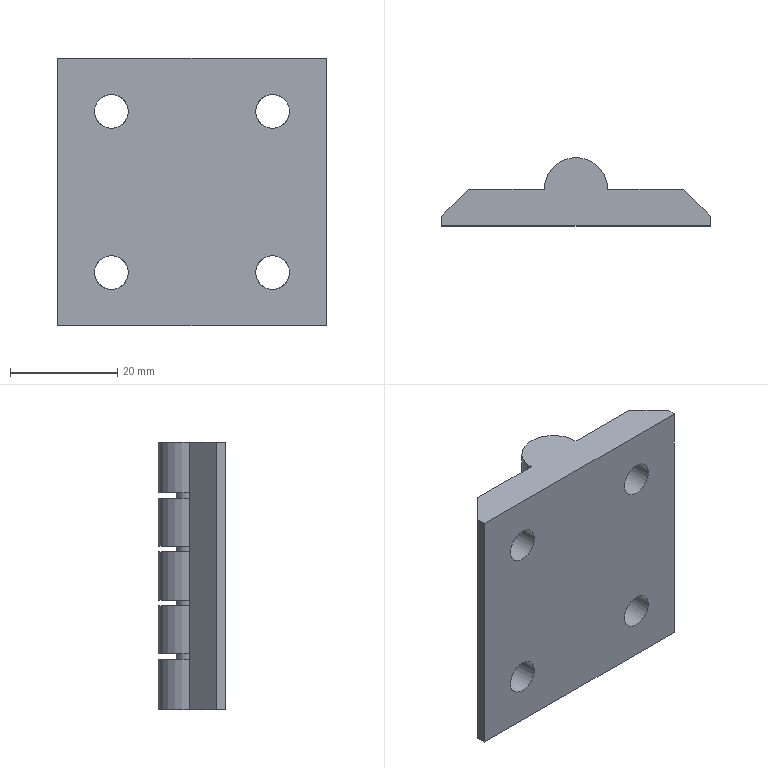Part | STEP file | 冲床-300配套压波_id422_x_t | 1 solid | 34 faces | box 50 x 12.7 x 49.8 mm | volume 17221 mm3 | plane 17 | cylinder 13 | cone 4 | commonest cylinder face diameters 11.8 x5 5 x4 6.3 x4
STEP:
#1=CARTESIAN_POINT('',(1212.5,286.8,-679.6));
#2=VERTEX_POINT('',#1);
#3=CARTESIAN_POINT('',(1212.5,286.8,-680.6));
#4=VERTEX_POINT('',#3);
#5=CARTESIAN_POINT('',(1212.5,286.8,-684.2));
#6=DIRECTION('',(0.,0.,-1.));
#7=VECTOR('',#6,1.);
#8=LINE('',#5,#7);
#9=EDGE_CURVE('',#2,#4,#8,.T.);
#10=ORIENTED_EDGE('',*,*,#9,.F.);
#11=CARTESIAN_POINT('',(1215.9,286.8,-679.6));
#12=VERTEX_POINT('',#11);
#13=CARTESIAN_POINT('',(1220.025,286.8,-679.6));
#14=DIRECTION('',(1.,0.,0.));
#15=VECTOR('',#14,1.);
#16=LINE('',#13,#15);
#17=EDGE_CURVE('',#2,#12,#16,.T.);
#18=ORIENTED_EDGE('',*,*,#17,.T.);
#19=CARTESIAN_POINT('',(1215.9,286.8,-670.6));
#20=VERTEX_POINT('',#19);
#21=CARTESIAN_POINT('',(1215.9,286.8,-640.2));
#22=DIRECTION('',(0.,0.,1.));
#23=VECTOR('',#22,1.);
#24=LINE('',#21,#23);
#25=EDGE_CURVE('',#12,#20,#24,.T.);
#26=ORIENTED_EDGE('',*,*,#25,.T.);
#27=CARTESIAN_POINT('',(1212.5,286.8,-670.6));
#28=VERTEX_POINT('',#27);
#29=CARTESIAN_POINT('',(1195.667,286.8,-670.6));
#30=DIRECTION('',(-1.,0.,0.));
#31=VECTOR('',#30,1.);
#32=LINE('',#29,#31);
#33=EDGE_CURVE('',#20,#28,#32,.T.);
#34=ORIENTED_EDGE('',*,*,#33,.T.);
#35=CARTESIAN_POINT('',(1212.5,286.8,-669.6));
#36=VERTEX_POINT('',#35);
#37=CARTESIAN_POINT('',(1212.5,286.8,-684.2));
#38=DIRECTION('',(0.,0.,-1.));
#39=VECTOR('',#38,1.);
#40=LINE('',#37,#39);
#41=EDGE_CURVE('',#36,#28,#40,.T.);
#42=ORIENTED_EDGE('',*,*,#41,.F.);
#43=CARTESIAN_POINT('',(1215.9,286.8,-669.6));
#44=VERTEX_POINT('',#43);
#45=CARTESIAN_POINT('',(1220.025,286.8,-669.6));
#46=DIRECTION('',(1.,0.,0.));
#47=VECTOR('',#46,1.);
#48=LINE('',#45,#47);
#49=EDGE_CURVE('',#36,#44,#48,.T.);
#50=ORIENTED_EDGE('',*,*,#49,.T.);
#51=CARTESIAN_POINT('',(1215.9,286.8,-660.6));
#52=VERTEX_POINT('',#51);
#53=CARTESIAN_POINT('',(1215.9,286.8,-640.2));
#54=DIRECTION('',(0.,0.,1.));
#55=VECTOR('',#54,1.);
#56=LINE('',#53,#55);
#57=EDGE_CURVE('',#44,#52,#56,.T.);
#58=ORIENTED_EDGE('',*,*,#57,.T.);
#59=CARTESIAN_POINT('',(1212.5,286.8,-660.6));
#60=VERTEX_POINT('',#59);
#61=CARTESIAN_POINT('',(1195.667,286.8,-660.6));
#62=DIRECTION('',(-1.,0.,0.));
#63=VECTOR('',#62,1.);
#64=LINE('',#61,#63);
#65=EDGE_CURVE('',#52,#60,#64,.T.);
#66=ORIENTED_EDGE('',*,*,#65,.T.);
#67=CARTESIAN_POINT('',(1212.5,286.8,-659.6));
#68=VERTEX_POINT('',#67);
#69=CARTESIAN_POINT('',(1212.5,286.8,-684.2));
#70=DIRECTION('',(0.,0.,-1.));
#71=VECTOR('',#70,1.);
#72=LINE('',#69,#71);
#73=EDGE_CURVE('',#68,#60,#72,.T.);
#74=ORIENTED_EDGE('',*,*,#73,.F.);
#75=CARTESIAN_POINT('',(1215.9,286.8,-659.6));
#76=VERTEX_POINT('',#75);
#77=CARTESIAN_POINT('',(1220.025,286.8,-659.6));
#78=DIRECTION('',(1.,0.,0.));
#79=VECTOR('',#78,1.);
#80=LINE('',#77,#79);
#81=EDGE_CURVE('',#68,#76,#80,.T.);
#82=ORIENTED_EDGE('',*,*,#81,.T.);
#83=CARTESIAN_POINT('',(1215.9,286.8,-650.6));
#84=VERTEX_POINT('',#83);
#85=CARTESIAN_POINT('',(1215.9,286.8,-640.2));
#86=DIRECTION('',(0.,0.,1.));
#87=VECTOR('',#86,1.);
#88=LINE('',#85,#87);
#89=EDGE_CURVE('',#76,#84,#88,.T.);
#90=ORIENTED_EDGE('',*,*,#89,.T.);
#91=CARTESIAN_POINT('',(1212.5,286.8,-650.6));
#92=VERTEX_POINT('',#91);
#93=CARTESIAN_POINT('',(1195.667,286.8,-650.6));
#94=DIRECTION('',(-1.,0.,0.));
#95=VECTOR('',#94,1.);
#96=LINE('',#93,#95);
#97=EDGE_CURVE('',#84,#92,#96,.T.);
#98=ORIENTED_EDGE('',*,*,#97,.T.);
#99=CARTESIAN_POINT('',(1212.5,286.8,-649.6));
#100=VERTEX_POINT('',#99);
#101=CARTESIAN_POINT('',(1212.5,286.8,-684.2));
#102=DIRECTION('',(0.,0.,-1.));
#103=VECTOR('',#102,1.);
#104=LINE('',#101,#103);
#105=EDGE_CURVE('',#100,#92,#104,.T.);
#106=ORIENTED_EDGE('',*,*,#105,.F.);
#107=CARTESIAN_POINT('',(1215.9,286.8,-649.6));
#108=VERTEX_POINT('',#107);
#109=CARTESIAN_POINT('',(1220.025,286.8,-649.6));
#110=DIRECTION('',(1.,0.,0.));
#111=VECTOR('',#110,1.);
#112=LINE('',#109,#111);
#113=EDGE_CURVE('',#100,#108,#112,.T.);
#114=ORIENTED_EDGE('',*,*,#113,.T.);
#115=CARTESIAN_POINT('',(1215.9,286.8,-640.2));
#116=VERTEX_POINT('',#115);
#117=CARTESIAN_POINT('',(1215.9,286.8,-640.2));
#118=DIRECTION('',(0.,0.,1.));
#119=VECTOR('',#118,1.);
#120=LINE('',#117,#119);
#121=EDGE_CURVE('',#108,#116,#120,.T.);
#122=ORIENTED_EDGE('',*,*,#121,.T.);
#123=CARTESIAN_POINT('',(1230.,286.8,-640.2));
#124=VERTEX_POINT('',#123);
#125=CARTESIAN_POINT('',(1235.,286.8,-640.2));
#126=DIRECTION('',(1.,0.,0.));
#127=VECTOR('',#126,1.);
#128=LINE('',#125,#127);
#129=EDGE_CURVE('',#116,#124,#128,.T.);
#130=ORIENTED_EDGE('',*,*,#129,.T.);
#131=CARTESIAN_POINT('',(1230.,286.8,-650.1));
#132=VERTEX_POINT('',#131);
#133=CARTESIAN_POINT('',(1230.,286.8,-640.2));
#134=DIRECTION('',(0.,0.,-1.));
#135=VECTOR('',#134,1.);
#136=LINE('',#133,#135);
#137=EDGE_CURVE('',#124,#132,#136,.T.);
#138=ORIENTED_EDGE('',*,*,#137,.T.);
#139=CARTESIAN_POINT('',(1225.,286.8,-650.1));
#140=DIRECTION('',(0.,-1.,0.));
#141=DIRECTION('',(0.,0.,1.));
#142=AXIS2_PLACEMENT_3D('',#139,#140,#141);
#143=CIRCLE('',#142,5.);
#144=EDGE_CURVE('',#132,#132,#143,.T.);
#145=ORIENTED_EDGE('',*,*,#144,.T.);
#146=CARTESIAN_POINT('',(1230.,286.8,-680.1));
#147=VERTEX_POINT('',#146);
#148=CARTESIAN_POINT('',(1230.,286.8,-640.2));
#149=DIRECTION('',(0.,0.,-1.));
#150=VECTOR('',#149,1.);
#151=LINE('',#148,#150);
#152=EDGE_CURVE('',#132,#147,#151,.T.);
#153=ORIENTED_EDGE('',*,*,#152,.T.);
#154=CARTESIAN_POINT('',(1225.,286.8,-680.1));
#155=DIRECTION('',(0.,-1.,0.));
#156=DIRECTION('',(0.,0.,1.));
#157=AXIS2_PLACEMENT_3D('',#154,#155,#156);
#158=CIRCLE('',#157,5.);
#159=EDGE_CURVE('',#147,#147,#158,.T.);
#160=ORIENTED_EDGE('',*,*,#159,.T.);
#161=CARTESIAN_POINT('',(1230.,286.8,-690.));
#162=VERTEX_POINT('',#161);
#163=CARTESIAN_POINT('',(1230.,286.8,-640.2));
#164=DIRECTION('',(0.,0.,-1.));
#165=VECTOR('',#164,1.);
#166=LINE('',#163,#165);
#167=EDGE_CURVE('',#147,#162,#166,.T.);
#168=ORIENTED_EDGE('',*,*,#167,.T.);
#169=CARTESIAN_POINT('',(1215.9,286.8,-690.));
#170=VERTEX_POINT('',#169);
#171=CARTESIAN_POINT('',(1185.,286.8,-690.));
#172=DIRECTION('',(-1.,0.,0.));
#173=VECTOR('',#172,1.);
#174=LINE('',#171,#173);
#175=EDGE_CURVE('',#162,#170,#174,.T.);
#176=ORIENTED_EDGE('',*,*,#175,.T.);
#177=CARTESIAN_POINT('',(1215.9,286.8,-680.6));
#178=VERTEX_POINT('',#177);
#179=CARTESIAN_POINT('',(1215.9,286.8,-640.2));
#180=DIRECTION('',(0.,0.,1.));
#181=VECTOR('',#180,1.);
#182=LINE('',#179,#181);
#183=EDGE_CURVE('',#170,#178,#182,.T.);
#184=ORIENTED_EDGE('',*,*,#183,.T.);
#185=CARTESIAN_POINT('',(1195.667,286.8,-680.6));
#186=DIRECTION('',(-1.,0.,0.));
#187=VECTOR('',#186,1.);
#188=LINE('',#185,#187);
#189=EDGE_CURVE('',#178,#4,#188,.T.);
#190=ORIENTED_EDGE('',*,*,#189,.T.);
#191=EDGE_LOOP('',(#10,#18,#26,#34,#42,#50,#58,#66,#74,#82,#90,#98,#106,#114,#122,#130,#138,#145,#153,#160,#168,#176,#184,#190));
#192=FACE_OUTER_BOUND('',#191,.T.);
#193=CARTESIAN_POINT('',(804.448,286.8,-553.819));
#194=DIRECTION('',(0.,1.,0.));
#195=DIRECTION('',(0.,0.,-1.));
#196=AXIS2_PLACEMENT_3D('',#193,#194,#195);
#197=PLANE('',#196);
#198=ADVANCED_FACE('',(#192),#197,.T.);
#199=CARTESIAN_POINT('',(1204.1,286.8,-680.6));
#200=VERTEX_POINT('',#199);
#201=CARTESIAN_POINT('',(1210.,286.8,-680.6));
#202=DIRECTION('',(0.,0.,1.));
#203=DIRECTION('',(1.,0.,0.));
#204=AXIS2_PLACEMENT_3D('',#201,#202,#203);
#205=CIRCLE('',#204,5.9);
#206=EDGE_CURVE('',#178,#200,#205,.T.);
#207=ORIENTED_EDGE('',*,*,#206,.F.);
#208=ORIENTED_EDGE('',*,*,#183,.F.);
#209=CARTESIAN_POINT('',(1204.1,286.8,-690.));
#210=VERTEX_POINT('',#209);
#211=CARTESIAN_POINT('',(1210.,286.8,-690.));
#212=DIRECTION('',(0.,0.,-1.));
#213=DIRECTION('',(-1.,0.,0.));
#214=AXIS2_PLACEMENT_3D('',#211,#212,#213);
#215=CIRCLE('',#214,5.9);
#216=EDGE_CURVE('',#210,#170,#215,.T.);
#217=ORIENTED_EDGE('',*,*,#216,.F.);
#218=CARTESIAN_POINT('',(1204.1,286.8,-640.2));
#219=DIRECTION('',(0.,0.,-1.));
#220=VECTOR('',#219,1.);
#221=LINE('',#218,#220);
#222=EDGE_CURVE('',#200,#210,#221,.T.);
#223=ORIENTED_EDGE('',*,*,#222,.F.);
#224=EDGE_LOOP('',(#207,#208,#217,#223));
#225=FACE_OUTER_BOUND('',#224,.T.);
#226=CARTESIAN_POINT('',(1210.,286.8,-640.2));
#227=DIRECTION('',(0.,0.,-1.));
#228=DIRECTION('',(-1.,0.,0.));
#229=AXIS2_PLACEMENT_3D('',#226,#227,#228);
#230=CYLINDRICAL_SURFACE('',#229,5.9);
#231=ADVANCED_FACE('',(#225),#230,.T.);
#232=CARTESIAN_POINT('',(1204.1,286.8,-679.6));
#233=VERTEX_POINT('',#232);
#234=CARTESIAN_POINT('',(1210.,286.8,-679.6));
#235=DIRECTION('',(0.,0.,-1.));
#236=DIRECTION('',(-1.,0.,0.));
#237=AXIS2_PLACEMENT_3D('',#234,#235,#236);
#238=CIRCLE('',#237,5.9);
#239=EDGE_CURVE('',#233,#12,#238,.T.);
#240=ORIENTED_EDGE('',*,*,#239,.F.);
#241=CARTESIAN_POINT('',(1204.1,286.8,-670.6));
#242=VERTEX_POINT('',#241);
#243=CARTESIAN_POINT('',(1204.1,286.8,-640.2));
#244=DIRECTION('',(0.,0.,-1.));
#245=VECTOR('',#244,1.);
#246=LINE('',#243,#245);
#247=EDGE_CURVE('',#242,#233,#246,.T.);
#248=ORIENTED_EDGE('',*,*,#247,.F.);
#249=CARTESIAN_POINT('',(1210.,286.8,-670.6));
#250=DIRECTION('',(0.,0.,1.));
#251=DIRECTION('',(1.,0.,0.));
#252=AXIS2_PLACEMENT_3D('',#249,#250,#251);
#253=CIRCLE('',#252,5.9);
#254=EDGE_CURVE('',#20,#242,#253,.T.);
#255=ORIENTED_EDGE('',*,*,#254,.F.);
#256=ORIENTED_EDGE('',*,*,#25,.F.);
#257=EDGE_LOOP('',(#240,#248,#255,#256));
#258=FACE_OUTER_BOUND('',#257,.T.);
#259=CARTESIAN_POINT('',(1210.,286.8,-640.2));
#260=DIRECTION('',(0.,0.,-1.));
#261=DIRECTION('',(-1.,0.,0.));
#262=AXIS2_PLACEMENT_3D('',#259,#260,#261);
#263=CYLINDRICAL_SURFACE('',#262,5.9);
#264=ADVANCED_FACE('',(#258),#263,.T.);
#265=CARTESIAN_POINT('',(1204.1,286.8,-669.6));
#266=VERTEX_POINT('',#265);
#267=CARTESIAN_POINT('',(1210.,286.8,-669.6));
#268=DIRECTION('',(0.,0.,-1.));
#269=DIRECTION('',(-1.,0.,0.));
#270=AXIS2_PLACEMENT_3D('',#267,#268,#269);
#271=CIRCLE('',#270,5.9);
#272=EDGE_CURVE('',#266,#44,#271,.T.);
#273=ORIENTED_EDGE('',*,*,#272,.F.);
#274=CARTESIAN_POINT('',(1204.1,286.8,-660.6));
#275=VERTEX_POINT('',#274);
#276=CARTESIAN_POINT('',(1204.1,286.8,-640.2));
#277=DIRECTION('',(0.,0.,-1.));
#278=VECTOR('',#277,1.);
#279=LINE('',#276,#278);
#280=EDGE_CURVE('',#275,#266,#279,.T.);
#281=ORIENTED_EDGE('',*,*,#280,.F.);
#282=CARTESIAN_POINT('',(1210.,286.8,-660.6));
#283=DIRECTION('',(0.,0.,1.));
#284=DIRECTION('',(1.,0.,0.));
#285=AXIS2_PLACEMENT_3D('',#282,#283,#284);
#286=CIRCLE('',#285,5.9);
#287=EDGE_CURVE('',#52,#275,#286,.T.);
#288=ORIENTED_EDGE('',*,*,#287,.F.);
#289=ORIENTED_EDGE('',*,*,#57,.F.);
#290=EDGE_LOOP('',(#273,#281,#288,#289));
#291=FACE_OUTER_BOUND('',#290,.T.);
#292=CARTESIAN_POINT('',(1210.,286.8,-640.2));
#293=DIRECTION('',(0.,0.,-1.));
#294=DIRECTION('',(-1.,0.,0.));
#295=AXIS2_PLACEMENT_3D('',#292,#293,#294);
#296=CYLINDRICAL_SURFACE('',#295,5.9);
#297=ADVANCED_FACE('',(#291),#296,.T.);
#298=CARTESIAN_POINT('',(1204.1,286.8,-659.6));
#299=VERTEX_POINT('',#298);
#300=CARTESIAN_POINT('',(1210.,286.8,-659.6));
#301=DIRECTION('',(0.,0.,-1.));
#302=DIRECTION('',(-1.,0.,0.));
#303=AXIS2_PLACEMENT_3D('',#300,#301,#302);
#304=CIRCLE('',#303,5.9);
#305=EDGE_CURVE('',#299,#76,#304,.T.);
#306=ORIENTED_EDGE('',*,*,#305,.F.);
#307=CARTESIAN_POINT('',(1204.1,286.8,-650.6));
#308=VERTEX_POINT('',#307);
#309=CARTESIAN_POINT('',(1204.1,286.8,-640.2));
#310=DIRECTION('',(0.,0.,-1.));
#311=VECTOR('',#310,1.);
#312=LINE('',#309,#311);
#313=EDGE_CURVE('',#308,#299,#312,.T.);
#314=ORIENTED_EDGE('',*,*,#313,.F.);
#315=CARTESIAN_POINT('',(1210.,286.8,-650.6));
#316=DIRECTION('',(0.,0.,1.));
#317=DIRECTION('',(1.,0.,0.));
#318=AXIS2_PLACEMENT_3D('',#315,#316,#317);
#319=CIRCLE('',#318,5.9);
#320=EDGE_CURVE('',#84,#308,#319,.T.);
#321=ORIENTED_EDGE('',*,*,#320,.F.);
#322=ORIENTED_EDGE('',*,*,#89,.F.);
#323=EDGE_LOOP('',(#306,#314,#321,#322));
#324=FACE_OUTER_BOUND('',#323,.T.);
#325=CARTESIAN_POINT('',(1210.,286.8,-640.2));
#326=DIRECTION('',(0.,0.,-1.));
#327=DIRECTION('',(-1.,0.,0.));
#328=AXIS2_PLACEMENT_3D('',#325,#326,#327);
#329=CYLINDRICAL_SURFACE('',#328,5.9);
#330=ADVANCED_FACE('',(#324),#329,.T.);
#331=CARTESIAN_POINT('',(1204.1,286.8,-649.6));
#332=VERTEX_POINT('',#331);
#333=CARTESIAN_POINT('',(1210.,286.8,-649.6));
#334=DIRECTION('',(0.,0.,-1.));
#335=DIRECTION('',(-1.,0.,0.));
#336=AXIS2_PLACEMENT_3D('',#333,#334,#335);
#337=CIRCLE('',#336,5.9);
#338=EDGE_CURVE('',#332,#108,#337,.T.);
#339=ORIENTED_EDGE('',*,*,#338,.F.);
#340=CARTESIAN_POINT('',(1204.1,286.8,-640.2));
#341=VERTEX_POINT('',#340);
#342=CARTESIAN_POINT('',(1204.1,286.8,-640.2));
#343=DIRECTION('',(0.,0.,-1.));
#344=VECTOR('',#343,1.);
#345=LINE('',#342,#344);
#346=EDGE_CURVE('',#341,#332,#345,.T.);
#347=ORIENTED_EDGE('',*,*,#346,.F.);
#348=CARTESIAN_POINT('',(1210.,286.8,-640.2));
#349=DIRECTION('',(0.,0.,1.));
#350=DIRECTION('',(-1.,0.,0.));
#351=AXIS2_PLACEMENT_3D('',#348,#349,#350);
#352=CIRCLE('',#351,5.9);
#353=EDGE_CURVE('',#116,#341,#352,.T.);
#354=ORIENTED_EDGE('',*,*,#353,.F.);
#355=ORIENTED_EDGE('',*,*,#121,.F.);
#356=EDGE_LOOP('',(#339,#347,#354,#355));
#357=FACE_OUTER_BOUND('',#356,.T.);
#358=CARTESIAN_POINT('',(1210.,286.8,-640.2));
#359=DIRECTION('',(0.,0.,-1.));
#360=DIRECTION('',(-1.,0.,0.));
#361=AXIS2_PLACEMENT_3D('',#358,#359,#360);
#362=CYLINDRICAL_SURFACE('',#361,5.9);
#363=ADVANCED_FACE('',(#357),#362,.T.);
#364=CARTESIAN_POINT('',(1207.5,286.8,-650.6));
#365=VERTEX_POINT('',#364);
#366=CARTESIAN_POINT('',(1207.5,286.8,-649.6));
#367=VERTEX_POINT('',#366);
#368=CARTESIAN_POINT('',(1207.5,286.8,-684.2));
#369=DIRECTION('',(0.,0.,1.));
#370=VECTOR('',#369,1.);
#371=LINE('',#368,#370);
#372=EDGE_CURVE('',#365,#367,#371,.T.);
#373=ORIENTED_EDGE('',*,*,#372,.F.);
#374=CARTESIAN_POINT('',(1195.667,286.8,-650.6));
#375=DIRECTION('',(-1.,0.,0.));
#376=VECTOR('',#375,1.);
#377=LINE('',#374,#376);
#378=EDGE_CURVE('',#365,#308,#377,.T.);
#379=ORIENTED_EDGE('',*,*,#378,.T.);
#380=ORIENTED_EDGE('',*,*,#313,.T.);
#381=CARTESIAN_POINT('',(1207.5,286.8,-659.6));
#382=VERTEX_POINT('',#381);
#383=CARTESIAN_POINT('',(1220.025,286.8,-659.6));
#384=DIRECTION('',(1.,0.,0.));
#385=VECTOR('',#384,1.);
#386=LINE('',#383,#385);
#387=EDGE_CURVE('',#299,#382,#386,.T.);
#388=ORIENTED_EDGE('',*,*,#387,.T.);
#389=CARTESIAN_POINT('',(1207.5,286.8,-660.6));
#390=VERTEX_POINT('',#389);
#391=CARTESIAN_POINT('',(1207.5,286.8,-684.2));
#392=DIRECTION('',(0.,0.,1.));
#393=VECTOR('',#392,1.);
#394=LINE('',#391,#393);
#395=EDGE_CURVE('',#390,#382,#394,.T.);
#396=ORIENTED_EDGE('',*,*,#395,.F.);
#397=CARTESIAN_POINT('',(1195.667,286.8,-660.6));
#398=DIRECTION('',(-1.,0.,0.));
#399=VECTOR('',#398,1.);
#400=LINE('',#397,#399);
#401=EDGE_CURVE('',#390,#275,#400,.T.);
#402=ORIENTED_EDGE('',*,*,#401,.T.);
#403=ORIENTED_EDGE('',*,*,#280,.T.);
#404=CARTESIAN_POINT('',(1207.5,286.8,-669.6));
#405=VERTEX_POINT('',#404);
#406=CARTESIAN_POINT('',(1220.025,286.8,-669.6));
#407=DIRECTION('',(1.,0.,0.));
#408=VECTOR('',#407,1.);
#409=LINE('',#406,#408);
#410=EDGE_CURVE('',#266,#405,#409,.T.);
#411=ORIENTED_EDGE('',*,*,#410,.T.);
#412=CARTESIAN_POINT('',(1207.5,286.8,-670.6));
#413=VERTEX_POINT('',#412);
#414=CARTESIAN_POINT('',(1207.5,286.8,-684.2));
#415=DIRECTION('',(0.,0.,1.));
#416=VECTOR('',#415,1.);
#417=LINE('',#414,#416);
#418=EDGE_CURVE('',#413,#405,#417,.T.);
#419=ORIENTED_EDGE('',*,*,#418,.F.);
#420=CARTESIAN_POINT('',(1195.667,286.8,-670.6));
#421=DIRECTION('',(-1.,0.,0.));
#422=VECTOR('',#421,1.);
#423=LINE('',#420,#422);
#424=EDGE_CURVE('',#413,#242,#423,.T.);
#425=ORIENTED_EDGE('',*,*,#424,.T.);
#426=ORIENTED_EDGE('',*,*,#247,.T.);
#427=CARTESIAN_POINT('',(1207.5,286.8,-679.6));
#428=VERTEX_POINT('',#427);
#429=CARTESIAN_POINT('',(1220.025,286.8,-679.6));
#430=DIRECTION('',(1.,0.,0.));
#431=VECTOR('',#430,1.);
#432=LINE('',#429,#431);
#433=EDGE_CURVE('',#233,#428,#432,.T.);
#434=ORIENTED_EDGE('',*,*,#433,.T.);
#435=CARTESIAN_POINT('',(1207.5,286.8,-680.6));
#436=VERTEX_POINT('',#435);
#437=CARTESIAN_POINT('',(1207.5,286.8,-684.2));
#438=DIRECTION('',(0.,0.,1.));
#439=VECTOR('',#438,1.);
#440=LINE('',#437,#439);
#441=EDGE_CURVE('',#436,#428,#440,.T.);
#442=ORIENTED_EDGE('',*,*,#441,.F.);
#443=CARTESIAN_POINT('',(1195.667,286.8,-680.6));
#444=DIRECTION('',(-1.,0.,0.));
#445=VECTOR('',#444,1.);
#446=LINE('',#443,#445);
#447=EDGE_CURVE('',#436,#200,#446,.T.);
#448=ORIENTED_EDGE('',*,*,#447,.T.);
#449=ORIENTED_EDGE('',*,*,#222,.T.);
#450=CARTESIAN_POINT('',(1190.,286.8,-690.));
#451=VERTEX_POINT('',#450);
#452=CARTESIAN_POINT('',(1185.,286.8,-690.));
#453=DIRECTION('',(-1.,0.,0.));
#454=VECTOR('',#453,1.);
#455=LINE('',#452,#454);
#456=EDGE_CURVE('',#210,#451,#455,.T.);
#457=ORIENTED_EDGE('',*,*,#456,.T.);
#458=CARTESIAN_POINT('',(1190.,286.8,-680.1));
#459=VERTEX_POINT('',#458);
#460=CARTESIAN_POINT('',(1190.,286.8,-690.));
#461=DIRECTION('',(0.,0.,1.));
#462=VECTOR('',#461,1.);
#463=LINE('',#460,#462);
#464=EDGE_CURVE('',#451,#459,#463,.T.);
#465=ORIENTED_EDGE('',*,*,#464,.T.);
#466=CARTESIAN_POINT('',(1195.,286.8,-680.1));
#467=DIRECTION('',(0.,-1.,0.));
#468=DIRECTION('',(0.,0.,1.));
#469=AXIS2_PLACEMENT_3D('',#466,#467,#468);
#470=CIRCLE('',#469,5.);
#471=EDGE_CURVE('',#459,#459,#470,.T.);
#472=ORIENTED_EDGE('',*,*,#471,.T.);
#473=CARTESIAN_POINT('',(1190.,286.8,-650.1));
#474=VERTEX_POINT('',#473);
#475=CARTESIAN_POINT('',(1190.,286.8,-690.));
#476=DIRECTION('',(0.,0.,1.));
#477=VECTOR('',#476,1.);
#478=LINE('',#475,#477);
#479=EDGE_CURVE('',#459,#474,#478,.T.);
#480=ORIENTED_EDGE('',*,*,#479,.T.);
#481=CARTESIAN_POINT('',(1195.,286.8,-650.1));
#482=DIRECTION('',(0.,-1.,0.));
#483=DIRECTION('',(0.,0.,1.));
#484=AXIS2_PLACEMENT_3D('',#481,#482,#483);
#485=CIRCLE('',#484,5.);
#486=EDGE_CURVE('',#474,#474,#485,.T.);
#487=ORIENTED_EDGE('',*,*,#486,.T.);
#488=CARTESIAN_POINT('',(1190.,286.8,-640.2));
#489=VERTEX_POINT('',#488);
#490=CARTESIAN_POINT('',(1190.,286.8,-690.));
#491=DIRECTION('',(0.,0.,1.));
#492=VECTOR('',#491,1.);
#493=LINE('',#490,#492);
#494=EDGE_CURVE('',#474,#489,#493,.T.);
#495=ORIENTED_EDGE('',*,*,#494,.T.);
#496=CARTESIAN_POINT('',(1235.,286.8,-640.2));
#497=DIRECTION('',(1.,0.,0.));
#498=VECTOR('',#497,1.);
#499=LINE('',#496,#498);
#500=EDGE_CURVE('',#489,#341,#499,.T.);
#501=ORIENTED_EDGE('',*,*,#500,.T.);
#502=ORIENTED_EDGE('',*,*,#346,.T.);
#503=CARTESIAN_POINT('',(1220.025,286.8,-649.6));
#504=DIRECTION('',(1.,0.,0.));
#505=VECTOR('',#504,1.);
#506=LINE('',#503,#505);
#507=EDGE_CURVE('',#332,#367,#506,.T.);
#508=ORIENTED_EDGE('',*,*,#507,.T.);
#509=EDGE_LOOP('',(#373,#379,#380,#388,#396,#402,#403,#411,#419,#425,#426,#434,#442,#448,#449,#457,#465,#472,#480,#487,#495,#501,#502,#508));
#510=FACE_OUTER_BOUND('',#509,.T.);
#511=CARTESIAN_POINT('',(804.448,286.8,-553.819));
#512=DIRECTION('',(0.,1.,0.));
#513=DIRECTION('',(0.,0.,-1.));
#514=AXIS2_PLACEMENT_3D('',#511,#512,#513);
#515=PLANE('',#514);
#516=ADVANCED_FACE('',(#510),#515,.T.);
#517=CARTESIAN_POINT('',(1185.,280.,-690.));
#518=VERTEX_POINT('',#517);
#519=CARTESIAN_POINT('',(1185.,281.8,-690.));
#520=VERTEX_POINT('',#519);
#521=CARTESIAN_POINT('',(1185.,286.8,-690.));
#522=DIRECTION('',(0.,1.,0.));
#523=VECTOR('',#522,1.);
#524=LINE('',#521,#523);
#525=EDGE_CURVE('',#518,#520,#524,.T.);
#526=ORIENTED_EDGE('',*,*,#525,.F.);
#527=CARTESIAN_POINT('',(1185.,280.,-640.2));
#528=VERTEX_POINT('',#527);
#529=CARTESIAN_POINT('',(1185.,280.,-640.2));
#530=DIRECTION('',(0.,0.,1.));
#531=VECTOR('',#530,1.);
#532=LINE('',#529,#531);
#533=EDGE_CURVE('',#518,#528,#532,.T.);
#534=ORIENTED_EDGE('',*,*,#533,.T.);
#535=CARTESIAN_POINT('',(1185.,281.8,-640.2));
#536=VERTEX_POINT('',#535);
#537=CARTESIAN_POINT('',(1185.,286.8,-640.2));
#538=DIRECTION('',(0.,1.,0.));
#539=VECTOR('',#538,1.);
#540=LINE('',#537,#539);
#541=EDGE_CURVE('',#528,#536,#540,.T.);
#542=ORIENTED_EDGE('',*,*,#541,.T.);
#543=CARTESIAN_POINT('',(1185.,281.8,-640.2));
#544=DIRECTION('',(0.,0.,-1.));
#545=VECTOR('',#544,1.);
#546=LINE('',#543,#545);
#547=EDGE_CURVE('',#536,#520,#546,.T.);
#548=ORIENTED_EDGE('',*,*,#547,.T.);
#549=EDGE_LOOP('',(#526,#534,#542,#548));
#550=FACE_OUTER_BOUND('',#549,.T.);
#551=CARTESIAN_POINT('',(1185.,286.8,-640.2));
#552=DIRECTION('',(1.,0.,0.));
#553=DIRECTION('',(0.,0.,-1.));
#554=AXIS2_PLACEMENT_3D('',#551,#552,#553);
#555=PLANE('',#554);
#556=ADVANCED_FACE('',(#550),#555,.F.);
#557=CARTESIAN_POINT('',(1235.,280.,-690.));
#558=VERTEX_POINT('',#557);
#559=CARTESIAN_POINT('',(1235.,281.8,-690.));
#560=VERTEX_POINT('',#559);
#561=CARTESIAN_POINT('',(1235.,286.8,-690.));
#562=DIRECTION('',(0.,1.,0.));
#563=VECTOR('',#562,1.);
#564=LINE('',#561,#563);
#565=EDGE_CURVE('',#558,#560,#564,.T.);
#566=ORIENTED_EDGE('',*,*,#565,.F.);
#567=CARTESIAN_POINT('',(1210.,280.,-690.));
#568=DIRECTION('',(-1.,0.,0.));
#569=VECTOR('',#568,1.);
#570=LINE('',#567,#569);
#571=EDGE_CURVE('',#558,#518,#570,.T.);
#572=ORIENTED_EDGE('',*,*,#571,.T.);
#573=ORIENTED_EDGE('',*,*,#525,.T.);
#574=CARTESIAN_POINT('',(1190.,286.8,-690.));
#575=DIRECTION('',(0.7071,0.7071,0.));
#576=VECTOR('',#575,1.);
#577=LINE('',#574,#576);
#578=EDGE_CURVE('',#520,#451,#577,.T.);
#579=ORIENTED_EDGE('',*,*,#578,.T.);
#580=ORIENTED_EDGE('',*,*,#456,.F.);
#581=ORIENTED_EDGE('',*,*,#216,.T.);
#582=ORIENTED_EDGE('',*,*,#175,.F.);
#583=CARTESIAN_POINT('',(1230.,286.8,-690.));
#584=DIRECTION('',(0.7071,-0.7071,0.));
#585=VECTOR('',#584,1.);
#586=LINE('',#583,#585);
#587=EDGE_CURVE('',#162,#560,#586,.T.);
#588=ORIENTED_EDGE('',*,*,#587,.T.);
#589=EDGE_LOOP('',(#566,#572,#573,#579,#580,#581,#582,#588));
#590=FACE_OUTER_BOUND('',#589,.T.);
#591=CARTESIAN_POINT('',(1210.,286.8,-690.));
#592=DIRECTION('',(0.,0.,1.));
#593=DIRECTION('',(1.,0.,0.));
#594=AXIS2_PLACEMENT_3D('',#591,#592,#593);
#595=PLANE('',#594);
#596=ADVANCED_FACE('',(#590),#595,.F.);
#597=CARTESIAN_POINT('',(1235.,280.,-640.2));
#598=VERTEX_POINT('',#597);
#599=CARTESIAN_POINT('',(1235.,281.8,-640.2));
#600=VERTEX_POINT('',#599);
#601=CARTESIAN_POINT('',(1235.,286.8,-640.2));
#602=DIRECTION('',(0.,1.,0.));
#603=VECTOR('',#602,1.);
#604=LINE('',#601,#603);
#605=EDGE_CURVE('',#598,#600,#604,.T.);
#606=ORIENTED_EDGE('',*,*,#605,.F.);
#607=CARTESIAN_POINT('',(1235.,280.,-690.));
#608=DIRECTION('',(0.,0.,-1.));
#609=VECTOR('',#608,1.);
#610=LINE('',#607,#609);
#611=EDGE_CURVE('',#598,#558,#610,.T.);
#612=ORIENTED_EDGE('',*,*,#611,.T.);
#613=ORIENTED_EDGE('',*,*,#565,.T.);
#614=CARTESIAN_POINT('',(1235.,281.8,-690.));
#615=DIRECTION('',(0.,0.,1.));
#616=VECTOR('',#615,1.);
#617=LINE('',#614,#616);
#618=EDGE_CURVE('',#560,#600,#617,.T.);
#619=ORIENTED_EDGE('',*,*,#618,.T.);
#620=EDGE_LOOP('',(#606,#612,#613,#619));
#621=FACE_OUTER_BOUND('',#620,.T.);
#622=CARTESIAN_POINT('',(1235.,286.8,-690.));
#623=DIRECTION('',(-1.,0.,0.));
#624=DIRECTION('',(0.,0.,1.));
#625=AXIS2_PLACEMENT_3D('',#622,#623,#624);
#626=PLANE('',#625);
#627=ADVANCED_FACE('',(#621),#626,.F.);
#628=ORIENTED_EDGE('',*,*,#129,.F.);
#629=ORIENTED_EDGE('',*,*,#353,.T.);
#630=ORIENTED_EDGE('',*,*,#500,.F.);
#631=CARTESIAN_POINT('',(1190.,286.8,-640.2));
#632=DIRECTION('',(-0.7071,-0.7071,0.));
#633=VECTOR('',#632,1.);
#634=LINE('',#631,#633);
#635=EDGE_CURVE('',#489,#536,#634,.T.);
#636=ORIENTED_EDGE('',*,*,#635,.T.);
#637=ORIENTED_EDGE('',*,*,#541,.F.);
#638=CARTESIAN_POINT('',(1210.,280.,-640.2));
#639=DIRECTION('',(1.,0.,0.));
#640=VECTOR('',#639,1.);
#641=LINE('',#638,#640);
#642=EDGE_CURVE('',#528,#598,#641,.T.);
#643=ORIENTED_EDGE('',*,*,#642,.T.);
#644=ORIENTED_EDGE('',*,*,#605,.T.);
#645=CARTESIAN_POINT('',(1230.,286.8,-640.2));
#646=DIRECTION('',(-0.7071,0.7071,0.));
#647=VECTOR('',#646,1.);
#648=LINE('',#645,#647);
#649=EDGE_CURVE('',#600,#124,#648,.T.);
#650=ORIENTED_EDGE('',*,*,#649,.T.);
#651=EDGE_LOOP('',(#628,#629,#630,#636,#637,#643,#644,#650));
#652=FACE_OUTER_BOUND('',#651,.T.);
#653=CARTESIAN_POINT('',(1210.,286.8,-640.2));
#654=DIRECTION('',(0.,0.,-1.));
#655=DIRECTION('',(-1.,0.,0.));
#656=AXIS2_PLACEMENT_3D('',#653,#654,#655);
#657=PLANE('',#656);
#658=ADVANCED_FACE('',(#652),#657,.F.);
#659=CARTESIAN_POINT('',(1225.,280.,-683.25));
#660=VERTEX_POINT('',#659);
#661=CARTESIAN_POINT('',(1225.,280.,-680.1));
#662=DIRECTION('',(0.,1.,0.));
#663=DIRECTION('',(0.,0.,-1.));
#664=AXIS2_PLACEMENT_3D('',#661,#662,#663);
#665=CIRCLE('',#664,3.15);
#666=EDGE_CURVE('',#660,#660,#665,.T.);
#667=ORIENTED_EDGE('',*,*,#666,.T.);
#668=EDGE_LOOP('',(#667));
#669=FACE_BOUND('',#668,.T.);
#670=CARTESIAN_POINT('',(1195.,280.,-683.25));
#671=VERTEX_POINT('',#670);
#672=CARTESIAN_POINT('',(1195.,280.,-680.1));
#673=DIRECTION('',(0.,1.,0.));
#674=DIRECTION('',(0.,0.,-1.));
#675=AXIS2_PLACEMENT_3D('',#672,#673,#674);
#676=CIRCLE('',#675,3.15);
#677=EDGE_CURVE('',#671,#671,#676,.T.);
#678=ORIENTED_EDGE('',*,*,#677,.T.);
#679=EDGE_LOOP('',(#678));
#680=FACE_BOUND('',#679,.T.);
#681=CARTESIAN_POINT('',(1225.,280.,-653.25));
#682=VERTEX_POINT('',#681);
#683=CARTESIAN_POINT('',(1225.,280.,-650.1));
#684=DIRECTION('',(0.,1.,0.));
#685=DIRECTION('',(0.,0.,-1.));
#686=AXIS2_PLACEMENT_3D('',#683,#684,#685);
#687=CIRCLE('',#686,3.15);
#688=EDGE_CURVE('',#682,#682,#687,.T.);
#689=ORIENTED_EDGE('',*,*,#688,.T.);
#690=EDGE_LOOP('',(#689));
#691=FACE_BOUND('',#690,.T.);
#692=CARTESIAN_POINT('',(1195.,280.,-653.25));
#693=VERTEX_POINT('',#692);
#694=CARTESIAN_POINT('',(1195.,280.,-650.1));
#695=DIRECTION('',(0.,1.,0.));
#696=DIRECTION('',(0.,0.,-1.));
#697=AXIS2_PLACEMENT_3D('',#694,#695,#696);
#698=CIRCLE('',#697,3.15);
#699=EDGE_CURVE('',#693,#693,#698,.T.);
#700=ORIENTED_EDGE('',*,*,#699,.T.);
#701=EDGE_LOOP('',(#700));
#702=FACE_BOUND('',#701,.T.);
#703=ORIENTED_EDGE('',*,*,#533,.F.);
#704=ORIENTED_EDGE('',*,*,#571,.F.);
#705=ORIENTED_EDGE('',*,*,#611,.F.);
#706=ORIENTED_EDGE('',*,*,#642,.F.);
#707=EDGE_LOOP('',(#703,#704,#705,#706));
#708=FACE_BOUND('',#707,.T.);
#709=CARTESIAN_POINT('',(804.448,280.,-553.819));
#710=DIRECTION('',(0.,1.,0.));
#711=DIRECTION('',(0.,0.,-1.));
#712=AXIS2_PLACEMENT_3D('',#709,#710,#711);
#713=PLANE('',#712);
#714=ADVANCED_FACE('',(#669,#680,#691,#702,#708),#713,.F.);
#715=ORIENTED_EDGE('',*,*,#587,.F.);
#716=ORIENTED_EDGE('',*,*,#167,.F.);
#717=ORIENTED_EDGE('',*,*,#152,.F.);
#718=ORIENTED_EDGE('',*,*,#137,.F.);
#719=ORIENTED_EDGE('',*,*,#649,.F.);
#720=ORIENTED_EDGE('',*,*,#618,.F.);
#721=EDGE_LOOP('',(#715,#716,#717,#718,#719,#720));
#722=FACE_OUTER_BOUND('',#721,.T.);
#723=CARTESIAN_POINT('',(1230.,286.8,-553.819));
#724=DIRECTION('',(0.7071,0.7071,0.));
#725=DIRECTION('',(0.,0.,-1.));
#726=AXIS2_PLACEMENT_3D('',#723,#724,#725);
#727=PLANE('',#726);
#728=ADVANCED_FACE('',(#722),#727,.T.);
#729=ORIENTED_EDGE('',*,*,#635,.F.);
#730=ORIENTED_EDGE('',*,*,#494,.F.);
#731=ORIENTED_EDGE('',*,*,#479,.F.);
#732=ORIENTED_EDGE('',*,*,#464,.F.);
#733=ORIENTED_EDGE('',*,*,#578,.F.);
#734=ORIENTED_EDGE('',*,*,#547,.F.);
#735=EDGE_LOOP('',(#729,#730,#731,#732,#733,#734));
#736=FACE_OUTER_BOUND('',#735,.T.);
#737=CARTESIAN_POINT('',(1190.,286.8,-553.819));
#738=DIRECTION('',(-0.7071,0.7071,0.));
#739=DIRECTION('',(0.,0.,1.));
#740=AXIS2_PLACEMENT_3D('',#737,#738,#739);
#741=PLANE('',#740);
#742=ADVANCED_FACE('',(#736),#741,.T.);
#743=CARTESIAN_POINT('',(1195.,284.95,-646.95));
#744=VERTEX_POINT('',#743);
#745=CARTESIAN_POINT('',(1195.,284.95,-650.1));
#746=DIRECTION('',(0.,1.,0.));
#747=DIRECTION('',(0.,0.,1.));
#748=AXIS2_PLACEMENT_3D('',#745,#746,#747);
#749=CIRCLE('',#748,3.15);
#750=EDGE_CURVE('',#744,#744,#749,.T.);
#751=ORIENTED_EDGE('',*,*,#750,.T.);
#752=EDGE_LOOP('',(#751));
#753=FACE_BOUND('',#752,.T.);
#754=ORIENTED_EDGE('',*,*,#699,.F.);
#755=EDGE_LOOP('',(#754));
#756=FACE_BOUND('',#755,.T.);
#757=CARTESIAN_POINT('',(1195.,236.8,-650.1));
#758=DIRECTION('',(0.,-1.,0.));
#759=DIRECTION('',(0.,0.,1.));
#760=AXIS2_PLACEMENT_3D('',#757,#758,#759);
#761=CYLINDRICAL_SURFACE('',#760,3.15);
#762=ADVANCED_FACE('',(#753,#756),#761,.F.);
#763=ORIENTED_EDGE('',*,*,#750,.F.);
#764=EDGE_LOOP('',(#763));
#765=FACE_BOUND('',#764,.T.);
#766=ORIENTED_EDGE('',*,*,#486,.F.);
#767=EDGE_LOOP('',(#766));
#768=FACE_BOUND('',#767,.T.);
#769=CARTESIAN_POINT('',(1195.,286.8,-650.1));
#770=DIRECTION('',(0.,1.,0.));
#771=DIRECTION('',(0.,0.,-1.));
#772=AXIS2_PLACEMENT_3D('',#769,#770,#771);
#773=CONICAL_SURFACE('',#772,5.,45.);
#774=ADVANCED_FACE('',(#765,#768),#773,.F.);
#775=CARTESIAN_POINT('',(1225.,284.95,-646.95));
#776=VERTEX_POINT('',#775);
#777=CARTESIAN_POINT('',(1225.,284.95,-650.1));
#778=DIRECTION('',(0.,1.,0.));
#779=DIRECTION('',(0.,0.,1.));
#780=AXIS2_PLACEMENT_3D('',#777,#778,#779);
#781=CIRCLE('',#780,3.15);
#782=EDGE_CURVE('',#776,#776,#781,.T.);
#783=ORIENTED_EDGE('',*,*,#782,.T.);
#784=EDGE_LOOP('',(#783));
#785=FACE_BOUND('',#784,.T.);
#786=ORIENTED_EDGE('',*,*,#688,.F.);
#787=EDGE_LOOP('',(#786));
#788=FACE_BOUND('',#787,.T.);
#789=CARTESIAN_POINT('',(1225.,236.8,-650.1));
#790=DIRECTION('',(0.,-1.,0.));
#791=DIRECTION('',(0.,0.,1.));
#792=AXIS2_PLACEMENT_3D('',#789,#790,#791);
#793=CYLINDRICAL_SURFACE('',#792,3.15);
#794=ADVANCED_FACE('',(#785,#788),#793,.F.);
#795=ORIENTED_EDGE('',*,*,#782,.F.);
#796=EDGE_LOOP('',(#795));
#797=FACE_BOUND('',#796,.T.);
#798=ORIENTED_EDGE('',*,*,#144,.F.);
#799=EDGE_LOOP('',(#798));
#800=FACE_BOUND('',#799,.T.);
#801=CARTESIAN_POINT('',(1225.,286.8,-650.1));
#802=DIRECTION('',(0.,1.,0.));
#803=DIRECTION('',(0.,0.,-1.));
#804=AXIS2_PLACEMENT_3D('',#801,#802,#803);
#805=CONICAL_SURFACE('',#804,5.,45.);
#806=ADVANCED_FACE('',(#797,#800),#805,.F.);
#807=CARTESIAN_POINT('',(1195.,284.95,-676.95));
#808=VERTEX_POINT('',#807);
#809=CARTESIAN_POINT('',(1195.,284.95,-680.1));
#810=DIRECTION('',(0.,1.,0.));
#811=DIRECTION('',(0.,0.,1.));
#812=AXIS2_PLACEMENT_3D('',#809,#810,#811);
#813=CIRCLE('',#812,3.15);
#814=EDGE_CURVE('',#808,#808,#813,.T.);
#815=ORIENTED_EDGE('',*,*,#814,.T.);
#816=EDGE_LOOP('',(#815));
#817=FACE_BOUND('',#816,.T.);
#818=ORIENTED_EDGE('',*,*,#677,.F.);
#819=EDGE_LOOP('',(#818));
#820=FACE_BOUND('',#819,.T.);
#821=CARTESIAN_POINT('',(1195.,236.8,-680.1));
#822=DIRECTION('',(0.,-1.,0.));
#823=DIRECTION('',(0.,0.,1.));
#824=AXIS2_PLACEMENT_3D('',#821,#822,#823);
#825=CYLINDRICAL_SURFACE('',#824,3.15);
#826=ADVANCED_FACE('',(#817,#820),#825,.F.);
#827=ORIENTED_EDGE('',*,*,#814,.F.);
#828=EDGE_LOOP('',(#827));
#829=FACE_BOUND('',#828,.T.);
#830=ORIENTED_EDGE('',*,*,#471,.F.);
#831=EDGE_LOOP('',(#830));
#832=FACE_BOUND('',#831,.T.);
#833=CARTESIAN_POINT('',(1195.,286.8,-680.1));
#834=DIRECTION('',(0.,1.,0.));
#835=DIRECTION('',(0.,0.,-1.));
#836=AXIS2_PLACEMENT_3D('',#833,#834,#835);
#837=CONICAL_SURFACE('',#836,5.,45.);
#838=ADVANCED_FACE('',(#829,#832),#837,.F.);
#839=CARTESIAN_POINT('',(1225.,284.95,-676.95));
#840=VERTEX_POINT('',#839);
#841=CARTESIAN_POINT('',(1225.,284.95,-680.1));
#842=DIRECTION('',(0.,1.,0.));
#843=DIRECTION('',(0.,0.,1.));
#844=AXIS2_PLACEMENT_3D('',#841,#842,#843);
#845=CIRCLE('',#844,3.15);
#846=EDGE_CURVE('',#840,#840,#845,.T.);
#847=ORIENTED_EDGE('',*,*,#846,.T.);
#848=EDGE_LOOP('',(#847));
#849=FACE_BOUND('',#848,.T.);
#850=ORIENTED_EDGE('',*,*,#666,.F.);
#851=EDGE_LOOP('',(#850));
#852=FACE_BOUND('',#851,.T.);
#853=CARTESIAN_POINT('',(1225.,236.8,-680.1));
#854=DIRECTION('',(0.,-1.,0.));
#855=DIRECTION('',(0.,0.,1.));
#856=AXIS2_PLACEMENT_3D('',#853,#854,#855);
#857=CYLINDRICAL_SURFACE('',#856,3.15);
#858=ADVANCED_FACE('',(#849,#852),#857,.F.);
#859=ORIENTED_EDGE('',*,*,#846,.F.);
#860=EDGE_LOOP('',(#859));
#861=FACE_BOUND('',#860,.T.);
#862=ORIENTED_EDGE('',*,*,#159,.F.);
#863=EDGE_LOOP('',(#862));
#864=FACE_BOUND('',#863,.T.);
#865=CARTESIAN_POINT('',(1225.,286.8,-680.1));
#866=DIRECTION('',(0.,1.,0.));
#867=DIRECTION('',(0.,0.,-1.));
#868=AXIS2_PLACEMENT_3D('',#865,#866,#867);
#869=CONICAL_SURFACE('',#868,5.,45.);
#870=ADVANCED_FACE('',(#861,#864),#869,.F.);
#871=CARTESIAN_POINT('',(1210.,286.8,-650.6));
#872=DIRECTION('',(0.,0.,1.));
#873=DIRECTION('',(1.,0.,0.));
#874=AXIS2_PLACEMENT_3D('',#871,#872,#873);
#875=CIRCLE('',#874,2.5);
#876=EDGE_CURVE('',#92,#365,#875,.T.);
#877=ORIENTED_EDGE('',*,*,#876,.F.);
#878=ORIENTED_EDGE('',*,*,#97,.F.);
#879=ORIENTED_EDGE('',*,*,#320,.T.);
#880=ORIENTED_EDGE('',*,*,#378,.F.);
#881=EDGE_LOOP('',(#877,#878,#879,#880));
#882=FACE_OUTER_BOUND('',#881,.T.);
#883=CARTESIAN_POINT('',(1195.667,330.8,-650.6));
#884=DIRECTION('',(0.,0.,1.));
#885=DIRECTION('',(1.,0.,0.));
#886=AXIS2_PLACEMENT_3D('',#883,#884,#885);
#887=PLANE('',#886);
#888=ADVANCED_FACE('',(#882),#887,.T.);
#889=CARTESIAN_POINT('',(1210.,286.8,-649.6));
#890=DIRECTION('',(0.,0.,-1.));
#891=DIRECTION('',(-1.,0.,0.));
#892=AXIS2_PLACEMENT_3D('',#889,#890,#891);
#893=CIRCLE('',#892,2.5);
#894=EDGE_CURVE('',#367,#100,#893,.T.);
#895=ORIENTED_EDGE('',*,*,#894,.F.);
#896=ORIENTED_EDGE('',*,*,#507,.F.);
#897=ORIENTED_EDGE('',*,*,#338,.T.);
#898=ORIENTED_EDGE('',*,*,#113,.F.);
#899=EDGE_LOOP('',(#895,#896,#897,#898));
#900=FACE_OUTER_BOUND('',#899,.T.);
#901=CARTESIAN_POINT('',(1220.025,330.8,-649.6));
#902=DIRECTION('',(0.,0.,-1.));
#903=DIRECTION('',(-1.,0.,0.));
#904=AXIS2_PLACEMENT_3D('',#901,#902,#903);
#905=PLANE('',#904);
#906=ADVANCED_FACE('',(#900),#905,.T.);
#907=CARTESIAN_POINT('',(1210.,286.8,-660.6));
#908=DIRECTION('',(0.,0.,1.));
#909=DIRECTION('',(1.,0.,0.));
#910=AXIS2_PLACEMENT_3D('',#907,#908,#909);
#911=CIRCLE('',#910,2.5);
#912=EDGE_CURVE('',#60,#390,#911,.T.);
#913=ORIENTED_EDGE('',*,*,#912,.F.);
#914=ORIENTED_EDGE('',*,*,#65,.F.);
#915=ORIENTED_EDGE('',*,*,#287,.T.);
#916=ORIENTED_EDGE('',*,*,#401,.F.);
#917=EDGE_LOOP('',(#913,#914,#915,#916));
#918=FACE_OUTER_BOUND('',#917,.T.);
#919=CARTESIAN_POINT('',(1195.667,330.8,-660.6));
#920=DIRECTION('',(0.,0.,1.));
#921=DIRECTION('',(1.,0.,0.));
#922=AXIS2_PLACEMENT_3D('',#919,#920,#921);
#923=PLANE('',#922);
#924=ADVANCED_FACE('',(#918),#923,.T.);
#925=CARTESIAN_POINT('',(1210.,286.8,-659.6));
#926=DIRECTION('',(0.,0.,-1.));
#927=DIRECTION('',(-1.,0.,0.));
#928=AXIS2_PLACEMENT_3D('',#925,#926,#927);
#929=CIRCLE('',#928,2.5);
#930=EDGE_CURVE('',#382,#68,#929,.T.);
#931=ORIENTED_EDGE('',*,*,#930,.F.);
#932=ORIENTED_EDGE('',*,*,#387,.F.);
#933=ORIENTED_EDGE('',*,*,#305,.T.);
#934=ORIENTED_EDGE('',*,*,#81,.F.);
#935=EDGE_LOOP('',(#931,#932,#933,#934));
#936=FACE_OUTER_BOUND('',#935,.T.);
#937=CARTESIAN_POINT('',(1220.025,330.8,-659.6));
#938=DIRECTION('',(0.,0.,-1.));
#939=DIRECTION('',(-1.,0.,0.));
#940=AXIS2_PLACEMENT_3D('',#937,#938,#939);
#941=PLANE('',#940);
#942=ADVANCED_FACE('',(#936),#941,.T.);
#943=CARTESIAN_POINT('',(1210.,286.8,-670.6));
#944=DIRECTION('',(0.,0.,1.));
#945=DIRECTION('',(1.,0.,0.));
#946=AXIS2_PLACEMENT_3D('',#943,#944,#945);
#947=CIRCLE('',#946,2.5);
#948=EDGE_CURVE('',#28,#413,#947,.T.);
#949=ORIENTED_EDGE('',*,*,#948,.F.);
#950=ORIENTED_EDGE('',*,*,#33,.F.);
#951=ORIENTED_EDGE('',*,*,#254,.T.);
#952=ORIENTED_EDGE('',*,*,#424,.F.);
#953=EDGE_LOOP('',(#949,#950,#951,#952));
#954=FACE_OUTER_BOUND('',#953,.T.);
#955=CARTESIAN_POINT('',(1195.667,330.8,-670.6));
#956=DIRECTION('',(0.,0.,1.));
#957=DIRECTION('',(1.,0.,0.));
#958=AXIS2_PLACEMENT_3D('',#955,#956,#957);
#959=PLANE('',#958);
#960=ADVANCED_FACE('',(#954),#959,.T.);
#961=CARTESIAN_POINT('',(1210.,286.8,-669.6));
#962=DIRECTION('',(0.,0.,-1.));
#963=DIRECTION('',(-1.,0.,0.));
#964=AXIS2_PLACEMENT_3D('',#961,#962,#963);
#965=CIRCLE('',#964,2.5);
#966=EDGE_CURVE('',#405,#36,#965,.T.);
#967=ORIENTED_EDGE('',*,*,#966,.F.);
#968=ORIENTED_EDGE('',*,*,#410,.F.);
#969=ORIENTED_EDGE('',*,*,#272,.T.);
#970=ORIENTED_EDGE('',*,*,#49,.F.);
#971=EDGE_LOOP('',(#967,#968,#969,#970));
#972=FACE_OUTER_BOUND('',#971,.T.);
#973=CARTESIAN_POINT('',(1220.025,330.8,-669.6));
#974=DIRECTION('',(0.,0.,-1.));
#975=DIRECTION('',(-1.,0.,0.));
#976=AXIS2_PLACEMENT_3D('',#973,#974,#975);
#977=PLANE('',#976);
#978=ADVANCED_FACE('',(#972),#977,.T.);
#979=CARTESIAN_POINT('',(1210.,286.8,-680.6));
#980=DIRECTION('',(0.,0.,1.));
#981=DIRECTION('',(1.,0.,0.));
#982=AXIS2_PLACEMENT_3D('',#979,#980,#981);
#983=CIRCLE('',#982,2.5);
#984=EDGE_CURVE('',#4,#436,#983,.T.);
#985=ORIENTED_EDGE('',*,*,#984,.F.);
#986=ORIENTED_EDGE('',*,*,#189,.F.);
#987=ORIENTED_EDGE('',*,*,#206,.T.);
#988=ORIENTED_EDGE('',*,*,#447,.F.);
#989=EDGE_LOOP('',(#985,#986,#987,#988));
#990=FACE_OUTER_BOUND('',#989,.T.);
#991=CARTESIAN_POINT('',(1195.667,330.8,-680.6));
#992=DIRECTION('',(0.,0.,1.));
#993=DIRECTION('',(1.,0.,0.));
#994=AXIS2_PLACEMENT_3D('',#991,#992,#993);
#995=PLANE('',#994);
#996=ADVANCED_FACE('',(#990),#995,.T.);
#997=CARTESIAN_POINT('',(1210.,286.8,-679.6));
#998=DIRECTION('',(0.,0.,-1.));
#999=DIRECTION('',(-1.,0.,0.));
#1000=AXIS2_PLACEMENT_3D('',#997,#998,#999);
#1001=CIRCLE('',#1000,2.5);
#1002=EDGE_CURVE('',#428,#2,#1001,.T.);
#1003=ORIENTED_EDGE('',*,*,#1002,.F.);
#1004=ORIENTED_EDGE('',*,*,#433,.F.);
#1005=ORIENTED_EDGE('',*,*,#239,.T.);
#1006=ORIENTED_EDGE('',*,*,#17,.F.);
#1007=EDGE_LOOP('',(#1003,#1004,#1005,#1006));
#1008=FACE_OUTER_BOUND('',#1007,.T.);
#1009=CARTESIAN_POINT('',(1220.025,330.8,-679.6));
#1010=DIRECTION('',(0.,0.,-1.));
#1011=DIRECTION('',(-1.,0.,0.));
#1012=AXIS2_PLACEMENT_3D('',#1009,#1010,#1011);
#1013=PLANE('',#1012);
#1014=ADVANCED_FACE('',(#1008),#1013,.T.);
#1015=ORIENTED_EDGE('',*,*,#441,.T.);
#1016=ORIENTED_EDGE('',*,*,#1002,.T.);
#1017=ORIENTED_EDGE('',*,*,#9,.T.);
#1018=ORIENTED_EDGE('',*,*,#984,.T.);
#1019=EDGE_LOOP('',(#1015,#1016,#1017,#1018));
#1020=FACE_OUTER_BOUND('',#1019,.T.);
#1021=CARTESIAN_POINT('',(1210.,286.8,-684.2));
#1022=DIRECTION('',(0.,0.,1.));
#1023=DIRECTION('',(1.,0.,0.));
#1024=AXIS2_PLACEMENT_3D('',#1021,#1022,#1023);
#1025=CYLINDRICAL_SURFACE('',#1024,2.5);
#1026=ADVANCED_FACE('',(#1020),#1025,.T.);
#1027=ORIENTED_EDGE('',*,*,#418,.T.);
#1028=ORIENTED_EDGE('',*,*,#966,.T.);
#1029=ORIENTED_EDGE('',*,*,#41,.T.);
#1030=ORIENTED_EDGE('',*,*,#948,.T.);
#1031=EDGE_LOOP('',(#1027,#1028,#1029,#1030));
#1032=FACE_OUTER_BOUND('',#1031,.T.);
#1033=CARTESIAN_POINT('',(1210.,286.8,-684.2));
#1034=DIRECTION('',(0.,0.,1.));
#1035=DIRECTION('',(1.,0.,0.));
#1036=AXIS2_PLACEMENT_3D('',#1033,#1034,#1035);
#1037=CYLINDRICAL_SURFACE('',#1036,2.5);
#1038=ADVANCED_FACE('',(#1032),#1037,.T.);
#1039=ORIENTED_EDGE('',*,*,#395,.T.);
#1040=ORIENTED_EDGE('',*,*,#930,.T.);
#1041=ORIENTED_EDGE('',*,*,#73,.T.);
#1042=ORIENTED_EDGE('',*,*,#912,.T.);
#1043=EDGE_LOOP('',(#1039,#1040,#1041,#1042));
#1044=FACE_OUTER_BOUND('',#1043,.T.);
#1045=CARTESIAN_POINT('',(1210.,286.8,-684.2));
#1046=DIRECTION('',(0.,0.,1.));
#1047=DIRECTION('',(1.,0.,0.));
#1048=AXIS2_PLACEMENT_3D('',#1045,#1046,#1047);
#1049=CYLINDRICAL_SURFACE('',#1048,2.5);
#1050=ADVANCED_FACE('',(#1044),#1049,.T.);
#1051=ORIENTED_EDGE('',*,*,#372,.T.);
#1052=ORIENTED_EDGE('',*,*,#894,.T.);
#1053=ORIENTED_EDGE('',*,*,#105,.T.);
#1054=ORIENTED_EDGE('',*,*,#876,.T.);
#1055=EDGE_LOOP('',(#1051,#1052,#1053,#1054));
#1056=FACE_OUTER_BOUND('',#1055,.T.);
#1057=CARTESIAN_POINT('',(1210.,286.8,-684.2));
#1058=DIRECTION('',(0.,0.,1.));
#1059=DIRECTION('',(1.,0.,0.));
#1060=AXIS2_PLACEMENT_3D('',#1057,#1058,#1059);
#1061=CYLINDRICAL_SURFACE('',#1060,2.5);
#1062=ADVANCED_FACE('',(#1056),#1061,.T.);
#1063=CLOSED_SHELL('',(#198,#231,#264,#297,#330,#363,#516,#556,#596,#627,#658,#714,#728,#742,#762,#774,#794,#806,#826,#838,#858,#870,#888,#906,#924,#942,#960,#978,#996,#1014,#1026,#1038,#1050,#1062));
#1064=MANIFOLD_SOLID_BREP('',#1063);
#1065=(LENGTH_UNIT()NAMED_UNIT(*)SI_UNIT(.MILLI.,.METRE.));
#1066=UNCERTAINTY_MEASURE_WITH_UNIT(LENGTH_MEASURE(0.00002),#1065,'','');
#1067=(NAMED_UNIT(*)PLANE_ANGLE_UNIT()SI_UNIT($,.RADIAN.));
#1068=PLANE_ANGLE_MEASURE_WITH_UNIT(PLANE_ANGLE_MEASURE(0.01745),#1067);
#1069=DIMENSIONAL_EXPONENTS(0.,0.,0.,0.,0.,0.,0.);
#1070=(CONVERSION_BASED_UNIT('DEGREE',#1068)NAMED_UNIT(#1069)PLANE_ANGLE_UNIT());
#1071=(NAMED_UNIT(*)SI_UNIT($,.STERADIAN.)SOLID_ANGLE_UNIT());
#1072=(GEOMETRIC_REPRESENTATION_CONTEXT(3)GLOBAL_UNCERTAINTY_ASSIGNED_CONTEXT((#1066))GLOBAL_UNIT_ASSIGNED_CONTEXT((#1065,#1070,#1071))REPRESENTATION_CONTEXT('',''));
#1073=ADVANCED_BREP_SHAPE_REPRESENTATION('',(#1064),#1072);